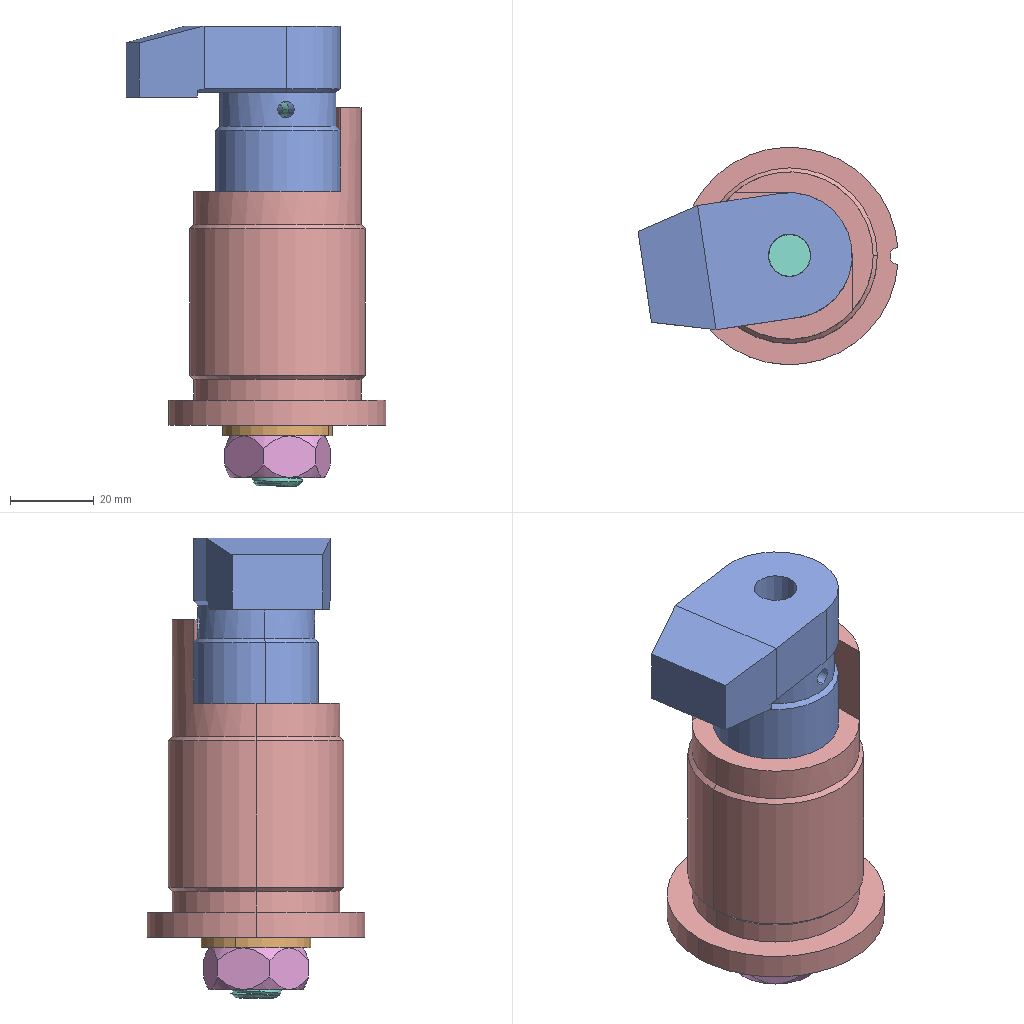Assembly | SolidWorks | 6 different items | 6 placed | box 62 x 52 x 110 mm
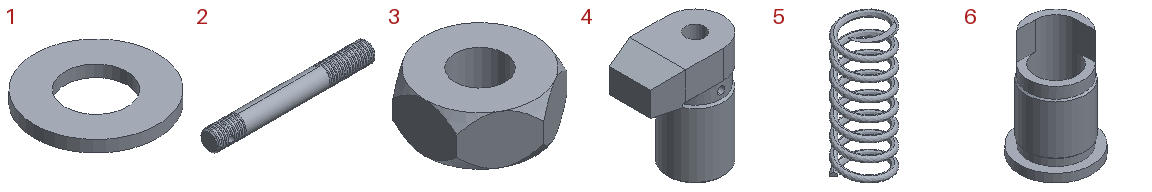Parts list (item | quantity | size | volume | features):
1 | x1 | 26.3 x 26.3 x 2.5 mm | 1016 mm3 | features Extrusion 1
2 | x1 | 98 x 12 x 12 mm | 10688 mm3 | features Helix 2, SweepCut 2, Chamfer 1, ICE 1, Revolution 1
3 | x1 | 22.517 x 26 x 10 mm | 3499 mm3 | features 3DProfileFeature 1, Extrusion 1, HoleWzd 1, ICE 1, MirrorPattern 1
4 | x1 | 50 x 30 x 60 mm | 40900 mm3 | features ICE 7, Chamfer 2, 3DProfileFeature 1, Extrusion 1, HoleWzd 1, MirrorPattern 1
5 | x1 | 17 x 17 x 46 mm | 1130 mm3 | features Helix 1, ICE 1, Sweep 1
6 | x1 | 51.923 x 52 x 76 mm | 55221 mm3 | features ICE 8, Chamfer 3, Extrusion 1
Mates (type | each side: item.copy, entity, surface, feature):
Concentric | 6.1 face cylinder Cut-Extrude4 | 2.1 face cylinder Revolve1
Concentric | 2.1 face cylinder Revolve1 | 1.1 face cylinder Boss-Extrude1
Coincident | 6.1 face plane Boss-Extrude1 | 1.1 face plane Boss-Extrude1
Concentric | 3.1 face cylinder M12 Tapped Hole3 | 2.1 face cylinder Revolve1
Coincident | 3.1 face plane Boss-Extrude1 | 1.1 face plane Boss-Extrude1
Tangent | 5.1 face surface:4006 Sweep1 | 2.1 face cylinder Revolve1
Coincident | 6.1 face plane Cut-Extrude2 | 5.1 face plane Cut-Extrude1
Concentric | 6.1 face cylinder Cut-Extrude2 | 4.1 face cylinder Cut-Extrude4
Concentric | 4.1 face cylinder Cut-Extrude5 | 2.1 face cylinder Cut-Extrude1
DistanceDim | 2.1 face plane Revolve1 | 3.1 face plane Boss-Extrude1